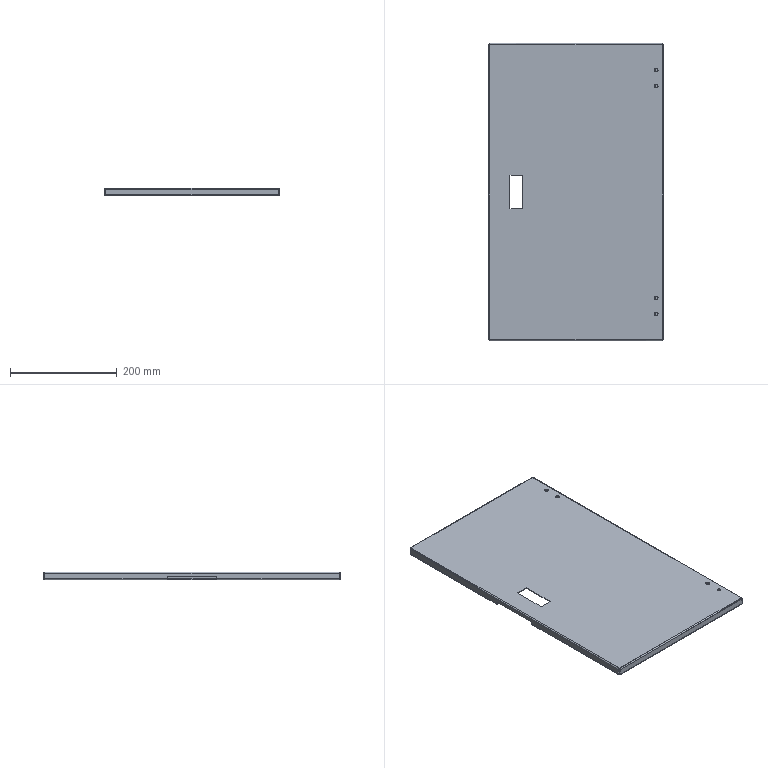Part | STEP file | 09-20 front door panel B (Default) | 1 solid | 90 faces | box 328 x 558 x 15 mm | volume 335829 mm3 | plane 48 | cylinder 26 | spline 16 | commonest cylinder face diameters 1.473 x9 4.473 x9 7 x8